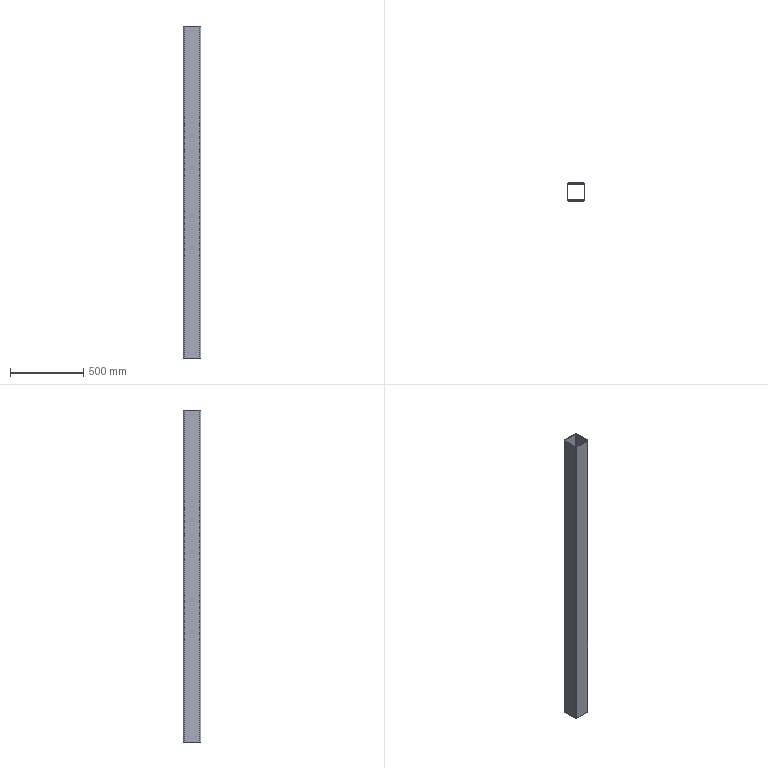Part | SolidWorks | features ICE 1, LibraryFeature 1 | 1 solid | 18 faces | box 120 x 120 x 2260 mm | volume 4101440 mm3 | plane 10 | cylinder 8 | commonest cylinder face diameters 8 x4 16 x4
STEP:
#1=CARTESIAN_POINT('',(52.,60.,-1130.));
#2=VERTEX_POINT('',#1);
#3=CARTESIAN_POINT('',(-52.,60.,-1130.));
#4=VERTEX_POINT('',#3);
#5=CARTESIAN_POINT('',(0.,60.,-1130.));
#6=DIRECTION('',(-1.,0.,0.));
#7=VECTOR('',#6,1000.);
#8=LINE('',#5,#7);
#9=EDGE_CURVE('',#2,#4,#8,.T.);
#10=ORIENTED_EDGE('',*,*,#9,.T.);
#11=CARTESIAN_POINT('',(-52.,60.,1130.));
#12=VERTEX_POINT('',#11);
#13=CARTESIAN_POINT('',(-52.,60.,1130.));
#14=DIRECTION('',(0.,0.,-1.));
#15=VECTOR('',#14,1000.);
#16=LINE('',#13,#15);
#17=EDGE_CURVE('',#12,#4,#16,.T.);
#18=ORIENTED_EDGE('',*,*,#17,.F.);
#19=CARTESIAN_POINT('',(52.,60.,1130.));
#20=VERTEX_POINT('',#19);
#21=CARTESIAN_POINT('',(0.,60.,1130.));
#22=DIRECTION('',(-1.,0.,0.));
#23=VECTOR('',#22,1000.);
#24=LINE('',#21,#23);
#25=EDGE_CURVE('',#20,#12,#24,.T.);
#26=ORIENTED_EDGE('',*,*,#25,.F.);
#27=CARTESIAN_POINT('',(52.,60.,1130.));
#28=DIRECTION('',(0.,0.,-1.));
#29=VECTOR('',#28,1000.);
#30=LINE('',#27,#29);
#31=EDGE_CURVE('',#20,#2,#30,.T.);
#32=ORIENTED_EDGE('',*,*,#31,.T.);
#33=EDGE_LOOP('',(#10,#18,#26,#32));
#34=FACE_OUTER_BOUND('',#33,.T.);
#35=CARTESIAN_POINT('',(0.,60.,1130.));
#36=DIRECTION('',(0.,-1.,0.));
#37=DIRECTION('',(0.,0.,-1.));
#38=AXIS2_PLACEMENT_3D('',#35,#36,#37);
#39=PLANE('',#38);
#40=ADVANCED_FACE('',(#34),#39,.F.);
#41=CARTESIAN_POINT('',(-60.,52.,-1130.));
#42=VERTEX_POINT('',#41);
#43=CARTESIAN_POINT('',(-52.,52.,-1130.));
#44=DIRECTION('',(0.,0.,1.));
#45=DIRECTION('',(1.,0.,0.));
#46=AXIS2_PLACEMENT_3D('',#43,#44,#45);
#47=CIRCLE('',#46,8.);
#48=EDGE_CURVE('',#4,#42,#47,.T.);
#49=ORIENTED_EDGE('',*,*,#48,.T.);
#50=CARTESIAN_POINT('',(-60.,52.,1130.));
#51=VERTEX_POINT('',#50);
#52=CARTESIAN_POINT('',(-60.,52.,1130.));
#53=DIRECTION('',(0.,0.,-1.));
#54=VECTOR('',#53,1000.);
#55=LINE('',#52,#54);
#56=EDGE_CURVE('',#51,#42,#55,.T.);
#57=ORIENTED_EDGE('',*,*,#56,.F.);
#58=CARTESIAN_POINT('',(-52.,52.,1130.));
#59=DIRECTION('',(0.,0.,1.));
#60=DIRECTION('',(1.,0.,0.));
#61=AXIS2_PLACEMENT_3D('',#58,#59,#60);
#62=CIRCLE('',#61,8.);
#63=EDGE_CURVE('',#12,#51,#62,.T.);
#64=ORIENTED_EDGE('',*,*,#63,.F.);
#65=ORIENTED_EDGE('',*,*,#17,.T.);
#66=EDGE_LOOP('',(#49,#57,#64,#65));
#67=FACE_OUTER_BOUND('',#66,.T.);
#68=CARTESIAN_POINT('',(-52.,52.,1130.));
#69=DIRECTION('',(0.,0.,-1.));
#70=DIRECTION('',(-1.,0.,0.));
#71=AXIS2_PLACEMENT_3D('',#68,#69,#70);
#72=CYLINDRICAL_SURFACE('',#71,8.);
#73=ADVANCED_FACE('',(#67),#72,.T.);
#74=CARTESIAN_POINT('',(-60.,-52.,-1130.));
#75=VERTEX_POINT('',#74);
#76=CARTESIAN_POINT('',(-60.,0.,-1130.));
#77=DIRECTION('',(0.,1.,0.));
#78=VECTOR('',#77,1000.);
#79=LINE('',#76,#78);
#80=EDGE_CURVE('',#75,#42,#79,.T.);
#81=ORIENTED_EDGE('',*,*,#80,.F.);
#82=CARTESIAN_POINT('',(-60.,-52.,1130.));
#83=VERTEX_POINT('',#82);
#84=CARTESIAN_POINT('',(-60.,-52.,1130.));
#85=DIRECTION('',(0.,0.,-1.));
#86=VECTOR('',#85,1000.);
#87=LINE('',#84,#86);
#88=EDGE_CURVE('',#83,#75,#87,.T.);
#89=ORIENTED_EDGE('',*,*,#88,.F.);
#90=CARTESIAN_POINT('',(-60.,0.,1130.));
#91=DIRECTION('',(0.,1.,0.));
#92=VECTOR('',#91,1000.);
#93=LINE('',#90,#92);
#94=EDGE_CURVE('',#83,#51,#93,.T.);
#95=ORIENTED_EDGE('',*,*,#94,.T.);
#96=ORIENTED_EDGE('',*,*,#56,.T.);
#97=EDGE_LOOP('',(#81,#89,#95,#96));
#98=FACE_OUTER_BOUND('',#97,.T.);
#99=CARTESIAN_POINT('',(-60.,0.,1130.));
#100=DIRECTION('',(-1.,0.,0.));
#101=DIRECTION('',(0.,0.,1.));
#102=AXIS2_PLACEMENT_3D('',#99,#100,#101);
#103=PLANE('',#102);
#104=ADVANCED_FACE('',(#98),#103,.T.);
#105=CARTESIAN_POINT('',(-52.,-60.,-1130.));
#106=VERTEX_POINT('',#105);
#107=CARTESIAN_POINT('',(-52.,-52.,-1130.));
#108=DIRECTION('',(0.,0.,1.));
#109=DIRECTION('',(1.,0.,0.));
#110=AXIS2_PLACEMENT_3D('',#107,#108,#109);
#111=CIRCLE('',#110,8.);
#112=EDGE_CURVE('',#75,#106,#111,.T.);
#113=ORIENTED_EDGE('',*,*,#112,.T.);
#114=CARTESIAN_POINT('',(-52.,-60.,1130.));
#115=VERTEX_POINT('',#114);
#116=CARTESIAN_POINT('',(-52.,-60.,1130.));
#117=DIRECTION('',(0.,0.,-1.));
#118=VECTOR('',#117,1000.);
#119=LINE('',#116,#118);
#120=EDGE_CURVE('',#115,#106,#119,.T.);
#121=ORIENTED_EDGE('',*,*,#120,.F.);
#122=CARTESIAN_POINT('',(-52.,-52.,1130.));
#123=DIRECTION('',(0.,0.,1.));
#124=DIRECTION('',(1.,0.,0.));
#125=AXIS2_PLACEMENT_3D('',#122,#123,#124);
#126=CIRCLE('',#125,8.);
#127=EDGE_CURVE('',#83,#115,#126,.T.);
#128=ORIENTED_EDGE('',*,*,#127,.F.);
#129=ORIENTED_EDGE('',*,*,#88,.T.);
#130=EDGE_LOOP('',(#113,#121,#128,#129));
#131=FACE_OUTER_BOUND('',#130,.T.);
#132=CARTESIAN_POINT('',(-52.,-52.,1130.));
#133=DIRECTION('',(0.,0.,-1.));
#134=DIRECTION('',(-1.,0.,0.));
#135=AXIS2_PLACEMENT_3D('',#132,#133,#134);
#136=CYLINDRICAL_SURFACE('',#135,8.);
#137=ADVANCED_FACE('',(#131),#136,.T.);
#138=CARTESIAN_POINT('',(52.,-60.,-1130.));
#139=VERTEX_POINT('',#138);
#140=CARTESIAN_POINT('',(0.,-60.,-1130.));
#141=DIRECTION('',(1.,0.,0.));
#142=VECTOR('',#141,1000.);
#143=LINE('',#140,#142);
#144=EDGE_CURVE('',#106,#139,#143,.T.);
#145=ORIENTED_EDGE('',*,*,#144,.T.);
#146=CARTESIAN_POINT('',(52.,-60.,1130.));
#147=VERTEX_POINT('',#146);
#148=CARTESIAN_POINT('',(52.,-60.,1130.));
#149=DIRECTION('',(0.,0.,-1.));
#150=VECTOR('',#149,1000.);
#151=LINE('',#148,#150);
#152=EDGE_CURVE('',#147,#139,#151,.T.);
#153=ORIENTED_EDGE('',*,*,#152,.F.);
#154=CARTESIAN_POINT('',(0.,-60.,1130.));
#155=DIRECTION('',(1.,0.,0.));
#156=VECTOR('',#155,1000.);
#157=LINE('',#154,#156);
#158=EDGE_CURVE('',#115,#147,#157,.T.);
#159=ORIENTED_EDGE('',*,*,#158,.F.);
#160=ORIENTED_EDGE('',*,*,#120,.T.);
#161=EDGE_LOOP('',(#145,#153,#159,#160));
#162=FACE_OUTER_BOUND('',#161,.T.);
#163=CARTESIAN_POINT('',(0.,-60.,1130.));
#164=DIRECTION('',(0.,1.,0.));
#165=DIRECTION('',(0.,0.,1.));
#166=AXIS2_PLACEMENT_3D('',#163,#164,#165);
#167=PLANE('',#166);
#168=ADVANCED_FACE('',(#162),#167,.F.);
#169=CARTESIAN_POINT('',(60.,-52.,-1130.));
#170=VERTEX_POINT('',#169);
#171=CARTESIAN_POINT('',(52.,-52.,-1130.));
#172=DIRECTION('',(0.,0.,1.));
#173=DIRECTION('',(1.,0.,0.));
#174=AXIS2_PLACEMENT_3D('',#171,#172,#173);
#175=CIRCLE('',#174,8.);
#176=EDGE_CURVE('',#139,#170,#175,.T.);
#177=ORIENTED_EDGE('',*,*,#176,.T.);
#178=CARTESIAN_POINT('',(60.,-52.,1130.));
#179=VERTEX_POINT('',#178);
#180=CARTESIAN_POINT('',(60.,-52.,1130.));
#181=DIRECTION('',(0.,0.,-1.));
#182=VECTOR('',#181,1000.);
#183=LINE('',#180,#182);
#184=EDGE_CURVE('',#179,#170,#183,.T.);
#185=ORIENTED_EDGE('',*,*,#184,.F.);
#186=CARTESIAN_POINT('',(52.,-52.,1130.));
#187=DIRECTION('',(0.,0.,1.));
#188=DIRECTION('',(1.,0.,0.));
#189=AXIS2_PLACEMENT_3D('',#186,#187,#188);
#190=CIRCLE('',#189,8.);
#191=EDGE_CURVE('',#147,#179,#190,.T.);
#192=ORIENTED_EDGE('',*,*,#191,.F.);
#193=ORIENTED_EDGE('',*,*,#152,.T.);
#194=EDGE_LOOP('',(#177,#185,#192,#193));
#195=FACE_OUTER_BOUND('',#194,.T.);
#196=CARTESIAN_POINT('',(52.,-52.,1130.));
#197=DIRECTION('',(0.,0.,-1.));
#198=DIRECTION('',(-1.,0.,0.));
#199=AXIS2_PLACEMENT_3D('',#196,#197,#198);
#200=CYLINDRICAL_SURFACE('',#199,8.);
#201=ADVANCED_FACE('',(#195),#200,.T.);
#202=CARTESIAN_POINT('',(60.,52.,-1130.));
#203=VERTEX_POINT('',#202);
#204=CARTESIAN_POINT('',(60.,0.,-1130.));
#205=DIRECTION('',(0.,-1.,0.));
#206=VECTOR('',#205,1000.);
#207=LINE('',#204,#206);
#208=EDGE_CURVE('',#203,#170,#207,.T.);
#209=ORIENTED_EDGE('',*,*,#208,.F.);
#210=CARTESIAN_POINT('',(60.,52.,1130.));
#211=VERTEX_POINT('',#210);
#212=CARTESIAN_POINT('',(60.,52.,1130.));
#213=DIRECTION('',(0.,0.,-1.));
#214=VECTOR('',#213,1000.);
#215=LINE('',#212,#214);
#216=EDGE_CURVE('',#211,#203,#215,.T.);
#217=ORIENTED_EDGE('',*,*,#216,.F.);
#218=CARTESIAN_POINT('',(60.,0.,1130.));
#219=DIRECTION('',(0.,-1.,0.));
#220=VECTOR('',#219,1000.);
#221=LINE('',#218,#220);
#222=EDGE_CURVE('',#211,#179,#221,.T.);
#223=ORIENTED_EDGE('',*,*,#222,.T.);
#224=ORIENTED_EDGE('',*,*,#184,.T.);
#225=EDGE_LOOP('',(#209,#217,#223,#224));
#226=FACE_OUTER_BOUND('',#225,.T.);
#227=CARTESIAN_POINT('',(60.,0.,1130.));
#228=DIRECTION('',(1.,0.,0.));
#229=DIRECTION('',(0.,0.,-1.));
#230=AXIS2_PLACEMENT_3D('',#227,#228,#229);
#231=PLANE('',#230);
#232=ADVANCED_FACE('',(#226),#231,.T.);
#233=CARTESIAN_POINT('',(-56.,-52.,-1130.));
#234=VERTEX_POINT('',#233);
#235=CARTESIAN_POINT('',(-52.,-56.,-1130.));
#236=VERTEX_POINT('',#235);
#237=CARTESIAN_POINT('',(-52.,-52.,-1130.));
#238=DIRECTION('',(0.,0.,1.));
#239=DIRECTION('',(1.,0.,0.));
#240=AXIS2_PLACEMENT_3D('',#237,#238,#239);
#241=CIRCLE('',#240,4.);
#242=EDGE_CURVE('',#234,#236,#241,.T.);
#243=ORIENTED_EDGE('',*,*,#242,.F.);
#244=CARTESIAN_POINT('',(-56.,-52.,1130.));
#245=VERTEX_POINT('',#244);
#246=CARTESIAN_POINT('',(-56.,-52.,1130.));
#247=DIRECTION('',(0.,0.,-1.));
#248=VECTOR('',#247,1000.);
#249=LINE('',#246,#248);
#250=EDGE_CURVE('',#245,#234,#249,.T.);
#251=ORIENTED_EDGE('',*,*,#250,.F.);
#252=CARTESIAN_POINT('',(-52.,-56.,1130.));
#253=VERTEX_POINT('',#252);
#254=CARTESIAN_POINT('',(-52.,-52.,1130.));
#255=DIRECTION('',(0.,0.,1.));
#256=DIRECTION('',(1.,0.,0.));
#257=AXIS2_PLACEMENT_3D('',#254,#255,#256);
#258=CIRCLE('',#257,4.);
#259=EDGE_CURVE('',#245,#253,#258,.T.);
#260=ORIENTED_EDGE('',*,*,#259,.T.);
#261=CARTESIAN_POINT('',(-52.,-56.,1130.));
#262=DIRECTION('',(0.,0.,-1.));
#263=VECTOR('',#262,1000.);
#264=LINE('',#261,#263);
#265=EDGE_CURVE('',#253,#236,#264,.T.);
#266=ORIENTED_EDGE('',*,*,#265,.T.);
#267=EDGE_LOOP('',(#243,#251,#260,#266));
#268=FACE_OUTER_BOUND('',#267,.T.);
#269=CARTESIAN_POINT('',(-52.,-52.,1130.));
#270=DIRECTION('',(0.,0.,-1.));
#271=DIRECTION('',(-1.,0.,0.));
#272=AXIS2_PLACEMENT_3D('',#269,#270,#271);
#273=CYLINDRICAL_SURFACE('',#272,4.);
#274=ADVANCED_FACE('',(#268),#273,.F.);
#275=CARTESIAN_POINT('',(-56.,52.,-1130.));
#276=VERTEX_POINT('',#275);
#277=CARTESIAN_POINT('',(-56.,0.,-1130.));
#278=DIRECTION('',(0.,1.,0.));
#279=VECTOR('',#278,1000.);
#280=LINE('',#277,#279);
#281=EDGE_CURVE('',#234,#276,#280,.T.);
#282=ORIENTED_EDGE('',*,*,#281,.T.);
#283=CARTESIAN_POINT('',(-56.,52.,1130.));
#284=VERTEX_POINT('',#283);
#285=CARTESIAN_POINT('',(-56.,52.,1130.));
#286=DIRECTION('',(0.,0.,-1.));
#287=VECTOR('',#286,1000.);
#288=LINE('',#285,#287);
#289=EDGE_CURVE('',#284,#276,#288,.T.);
#290=ORIENTED_EDGE('',*,*,#289,.F.);
#291=CARTESIAN_POINT('',(-56.,0.,1130.));
#292=DIRECTION('',(0.,1.,0.));
#293=VECTOR('',#292,1000.);
#294=LINE('',#291,#293);
#295=EDGE_CURVE('',#245,#284,#294,.T.);
#296=ORIENTED_EDGE('',*,*,#295,.F.);
#297=ORIENTED_EDGE('',*,*,#250,.T.);
#298=EDGE_LOOP('',(#282,#290,#296,#297));
#299=FACE_OUTER_BOUND('',#298,.T.);
#300=CARTESIAN_POINT('',(-56.,0.,1130.));
#301=DIRECTION('',(-1.,0.,0.));
#302=DIRECTION('',(0.,0.,1.));
#303=AXIS2_PLACEMENT_3D('',#300,#301,#302);
#304=PLANE('',#303);
#305=ADVANCED_FACE('',(#299),#304,.F.);
#306=CARTESIAN_POINT('',(-52.,56.,-1130.));
#307=VERTEX_POINT('',#306);
#308=CARTESIAN_POINT('',(-52.,52.,-1130.));
#309=DIRECTION('',(0.,0.,1.));
#310=DIRECTION('',(1.,0.,0.));
#311=AXIS2_PLACEMENT_3D('',#308,#309,#310);
#312=CIRCLE('',#311,4.);
#313=EDGE_CURVE('',#307,#276,#312,.T.);
#314=ORIENTED_EDGE('',*,*,#313,.F.);
#315=CARTESIAN_POINT('',(-52.,56.,1130.));
#316=VERTEX_POINT('',#315);
#317=CARTESIAN_POINT('',(-52.,56.,1130.));
#318=DIRECTION('',(0.,0.,-1.));
#319=VECTOR('',#318,1000.);
#320=LINE('',#317,#319);
#321=EDGE_CURVE('',#316,#307,#320,.T.);
#322=ORIENTED_EDGE('',*,*,#321,.F.);
#323=CARTESIAN_POINT('',(-52.,52.,1130.));
#324=DIRECTION('',(0.,0.,1.));
#325=DIRECTION('',(1.,0.,0.));
#326=AXIS2_PLACEMENT_3D('',#323,#324,#325);
#327=CIRCLE('',#326,4.);
#328=EDGE_CURVE('',#316,#284,#327,.T.);
#329=ORIENTED_EDGE('',*,*,#328,.T.);
#330=ORIENTED_EDGE('',*,*,#289,.T.);
#331=EDGE_LOOP('',(#314,#322,#329,#330));
#332=FACE_OUTER_BOUND('',#331,.T.);
#333=CARTESIAN_POINT('',(-52.,52.,1130.));
#334=DIRECTION('',(0.,0.,-1.));
#335=DIRECTION('',(-1.,0.,0.));
#336=AXIS2_PLACEMENT_3D('',#333,#334,#335);
#337=CYLINDRICAL_SURFACE('',#336,4.);
#338=ADVANCED_FACE('',(#332),#337,.F.);
#339=CARTESIAN_POINT('',(52.,56.,-1130.));
#340=VERTEX_POINT('',#339);
#341=CARTESIAN_POINT('',(0.,56.,-1130.));
#342=DIRECTION('',(-1.,0.,0.));
#343=VECTOR('',#342,1000.);
#344=LINE('',#341,#343);
#345=EDGE_CURVE('',#340,#307,#344,.T.);
#346=ORIENTED_EDGE('',*,*,#345,.F.);
#347=CARTESIAN_POINT('',(52.,56.,1130.));
#348=VERTEX_POINT('',#347);
#349=CARTESIAN_POINT('',(52.,56.,1130.));
#350=DIRECTION('',(0.,0.,-1.));
#351=VECTOR('',#350,1000.);
#352=LINE('',#349,#351);
#353=EDGE_CURVE('',#348,#340,#352,.T.);
#354=ORIENTED_EDGE('',*,*,#353,.F.);
#355=CARTESIAN_POINT('',(0.,56.,1130.));
#356=DIRECTION('',(-1.,0.,0.));
#357=VECTOR('',#356,1000.);
#358=LINE('',#355,#357);
#359=EDGE_CURVE('',#348,#316,#358,.T.);
#360=ORIENTED_EDGE('',*,*,#359,.T.);
#361=ORIENTED_EDGE('',*,*,#321,.T.);
#362=EDGE_LOOP('',(#346,#354,#360,#361));
#363=FACE_OUTER_BOUND('',#362,.T.);
#364=CARTESIAN_POINT('',(0.,56.,1130.));
#365=DIRECTION('',(0.,-1.,0.));
#366=DIRECTION('',(0.,0.,-1.));
#367=AXIS2_PLACEMENT_3D('',#364,#365,#366);
#368=PLANE('',#367);
#369=ADVANCED_FACE('',(#363),#368,.T.);
#370=CARTESIAN_POINT('',(56.,52.,-1130.));
#371=VERTEX_POINT('',#370);
#372=CARTESIAN_POINT('',(52.,52.,-1130.));
#373=DIRECTION('',(0.,0.,1.));
#374=DIRECTION('',(1.,0.,0.));
#375=AXIS2_PLACEMENT_3D('',#372,#373,#374);
#376=CIRCLE('',#375,4.);
#377=EDGE_CURVE('',#371,#340,#376,.T.);
#378=ORIENTED_EDGE('',*,*,#377,.F.);
#379=CARTESIAN_POINT('',(56.,52.,1130.));
#380=VERTEX_POINT('',#379);
#381=CARTESIAN_POINT('',(56.,52.,1130.));
#382=DIRECTION('',(0.,0.,-1.));
#383=VECTOR('',#382,1000.);
#384=LINE('',#381,#383);
#385=EDGE_CURVE('',#380,#371,#384,.T.);
#386=ORIENTED_EDGE('',*,*,#385,.F.);
#387=CARTESIAN_POINT('',(52.,52.,1130.));
#388=DIRECTION('',(0.,0.,1.));
#389=DIRECTION('',(1.,0.,0.));
#390=AXIS2_PLACEMENT_3D('',#387,#388,#389);
#391=CIRCLE('',#390,4.);
#392=EDGE_CURVE('',#380,#348,#391,.T.);
#393=ORIENTED_EDGE('',*,*,#392,.T.);
#394=ORIENTED_EDGE('',*,*,#353,.T.);
#395=EDGE_LOOP('',(#378,#386,#393,#394));
#396=FACE_OUTER_BOUND('',#395,.T.);
#397=CARTESIAN_POINT('',(52.,52.,1130.));
#398=DIRECTION('',(0.,0.,-1.));
#399=DIRECTION('',(-1.,0.,0.));
#400=AXIS2_PLACEMENT_3D('',#397,#398,#399);
#401=CYLINDRICAL_SURFACE('',#400,4.);
#402=ADVANCED_FACE('',(#396),#401,.F.);
#403=CARTESIAN_POINT('',(56.,-52.,-1130.));
#404=VERTEX_POINT('',#403);
#405=CARTESIAN_POINT('',(56.,0.,-1130.));
#406=DIRECTION('',(0.,-1.,0.));
#407=VECTOR('',#406,1000.);
#408=LINE('',#405,#407);
#409=EDGE_CURVE('',#371,#404,#408,.T.);
#410=ORIENTED_EDGE('',*,*,#409,.T.);
#411=CARTESIAN_POINT('',(56.,-52.,1130.));
#412=VERTEX_POINT('',#411);
#413=CARTESIAN_POINT('',(56.,-52.,1130.));
#414=DIRECTION('',(0.,0.,-1.));
#415=VECTOR('',#414,1000.);
#416=LINE('',#413,#415);
#417=EDGE_CURVE('',#412,#404,#416,.T.);
#418=ORIENTED_EDGE('',*,*,#417,.F.);
#419=CARTESIAN_POINT('',(56.,0.,1130.));
#420=DIRECTION('',(0.,-1.,0.));
#421=VECTOR('',#420,1000.);
#422=LINE('',#419,#421);
#423=EDGE_CURVE('',#380,#412,#422,.T.);
#424=ORIENTED_EDGE('',*,*,#423,.F.);
#425=ORIENTED_EDGE('',*,*,#385,.T.);
#426=EDGE_LOOP('',(#410,#418,#424,#425));
#427=FACE_OUTER_BOUND('',#426,.T.);
#428=CARTESIAN_POINT('',(56.,0.,1130.));
#429=DIRECTION('',(1.,0.,0.));
#430=DIRECTION('',(0.,0.,-1.));
#431=AXIS2_PLACEMENT_3D('',#428,#429,#430);
#432=PLANE('',#431);
#433=ADVANCED_FACE('',(#427),#432,.F.);
#434=CARTESIAN_POINT('',(52.,-56.,-1130.));
#435=VERTEX_POINT('',#434);
#436=CARTESIAN_POINT('',(52.,-52.,-1130.));
#437=DIRECTION('',(0.,0.,1.));
#438=DIRECTION('',(1.,0.,0.));
#439=AXIS2_PLACEMENT_3D('',#436,#437,#438);
#440=CIRCLE('',#439,4.);
#441=EDGE_CURVE('',#435,#404,#440,.T.);
#442=ORIENTED_EDGE('',*,*,#441,.F.);
#443=CARTESIAN_POINT('',(52.,-56.,1130.));
#444=VERTEX_POINT('',#443);
#445=CARTESIAN_POINT('',(52.,-56.,1130.));
#446=DIRECTION('',(0.,0.,-1.));
#447=VECTOR('',#446,1000.);
#448=LINE('',#445,#447);
#449=EDGE_CURVE('',#444,#435,#448,.T.);
#450=ORIENTED_EDGE('',*,*,#449,.F.);
#451=CARTESIAN_POINT('',(52.,-52.,1130.));
#452=DIRECTION('',(0.,0.,1.));
#453=DIRECTION('',(1.,0.,0.));
#454=AXIS2_PLACEMENT_3D('',#451,#452,#453);
#455=CIRCLE('',#454,4.);
#456=EDGE_CURVE('',#444,#412,#455,.T.);
#457=ORIENTED_EDGE('',*,*,#456,.T.);
#458=ORIENTED_EDGE('',*,*,#417,.T.);
#459=EDGE_LOOP('',(#442,#450,#457,#458));
#460=FACE_OUTER_BOUND('',#459,.T.);
#461=CARTESIAN_POINT('',(52.,-52.,1130.));
#462=DIRECTION('',(0.,0.,-1.));
#463=DIRECTION('',(-1.,0.,0.));
#464=AXIS2_PLACEMENT_3D('',#461,#462,#463);
#465=CYLINDRICAL_SURFACE('',#464,4.);
#466=ADVANCED_FACE('',(#460),#465,.F.);
#467=CARTESIAN_POINT('',(0.,-56.,-1130.));
#468=DIRECTION('',(1.,0.,0.));
#469=VECTOR('',#468,1000.);
#470=LINE('',#467,#469);
#471=EDGE_CURVE('',#236,#435,#470,.T.);
#472=ORIENTED_EDGE('',*,*,#471,.F.);
#473=ORIENTED_EDGE('',*,*,#265,.F.);
#474=CARTESIAN_POINT('',(0.,-56.,1130.));
#475=DIRECTION('',(1.,0.,0.));
#476=VECTOR('',#475,1000.);
#477=LINE('',#474,#476);
#478=EDGE_CURVE('',#253,#444,#477,.T.);
#479=ORIENTED_EDGE('',*,*,#478,.T.);
#480=ORIENTED_EDGE('',*,*,#449,.T.);
#481=EDGE_LOOP('',(#472,#473,#479,#480));
#482=FACE_OUTER_BOUND('',#481,.T.);
#483=CARTESIAN_POINT('',(0.,-56.,1130.));
#484=DIRECTION('',(0.,1.,0.));
#485=DIRECTION('',(0.,0.,1.));
#486=AXIS2_PLACEMENT_3D('',#483,#484,#485);
#487=PLANE('',#486);
#488=ADVANCED_FACE('',(#482),#487,.T.);
#489=CARTESIAN_POINT('',(52.,52.,-1130.));
#490=DIRECTION('',(0.,0.,1.));
#491=DIRECTION('',(1.,0.,0.));
#492=AXIS2_PLACEMENT_3D('',#489,#490,#491);
#493=CIRCLE('',#492,8.);
#494=EDGE_CURVE('',#203,#2,#493,.T.);
#495=ORIENTED_EDGE('',*,*,#494,.T.);
#496=ORIENTED_EDGE('',*,*,#31,.F.);
#497=CARTESIAN_POINT('',(52.,52.,1130.));
#498=DIRECTION('',(0.,0.,1.));
#499=DIRECTION('',(1.,0.,0.));
#500=AXIS2_PLACEMENT_3D('',#497,#498,#499);
#501=CIRCLE('',#500,8.);
#502=EDGE_CURVE('',#211,#20,#501,.T.);
#503=ORIENTED_EDGE('',*,*,#502,.F.);
#504=ORIENTED_EDGE('',*,*,#216,.T.);
#505=EDGE_LOOP('',(#495,#496,#503,#504));
#506=FACE_OUTER_BOUND('',#505,.T.);
#507=CARTESIAN_POINT('',(52.,52.,1130.));
#508=DIRECTION('',(0.,0.,-1.));
#509=DIRECTION('',(-1.,0.,0.));
#510=AXIS2_PLACEMENT_3D('',#507,#508,#509);
#511=CYLINDRICAL_SURFACE('',#510,8.);
#512=ADVANCED_FACE('',(#506),#511,.T.);
#513=ORIENTED_EDGE('',*,*,#259,.F.);
#514=ORIENTED_EDGE('',*,*,#295,.T.);
#515=ORIENTED_EDGE('',*,*,#328,.F.);
#516=ORIENTED_EDGE('',*,*,#359,.F.);
#517=ORIENTED_EDGE('',*,*,#392,.F.);
#518=ORIENTED_EDGE('',*,*,#423,.T.);
#519=ORIENTED_EDGE('',*,*,#456,.F.);
#520=ORIENTED_EDGE('',*,*,#478,.F.);
#521=EDGE_LOOP('',(#513,#514,#515,#516,#517,#518,#519,#520));
#522=FACE_BOUND('',#521,.T.);
#523=ORIENTED_EDGE('',*,*,#25,.T.);
#524=ORIENTED_EDGE('',*,*,#63,.T.);
#525=ORIENTED_EDGE('',*,*,#94,.F.);
#526=ORIENTED_EDGE('',*,*,#127,.T.);
#527=ORIENTED_EDGE('',*,*,#158,.T.);
#528=ORIENTED_EDGE('',*,*,#191,.T.);
#529=ORIENTED_EDGE('',*,*,#222,.F.);
#530=ORIENTED_EDGE('',*,*,#502,.T.);
#531=EDGE_LOOP('',(#523,#524,#525,#526,#527,#528,#529,#530));
#532=FACE_OUTER_BOUND('',#531,.T.);
#533=CARTESIAN_POINT('',(0.,0.,1130.));
#534=DIRECTION('',(0.,0.,1.));
#535=DIRECTION('',(1.,0.,0.));
#536=AXIS2_PLACEMENT_3D('',#533,#534,#535);
#537=PLANE('',#536);
#538=ADVANCED_FACE('',(#522,#532),#537,.T.);
#539=ORIENTED_EDGE('',*,*,#242,.T.);
#540=ORIENTED_EDGE('',*,*,#471,.T.);
#541=ORIENTED_EDGE('',*,*,#441,.T.);
#542=ORIENTED_EDGE('',*,*,#409,.F.);
#543=ORIENTED_EDGE('',*,*,#377,.T.);
#544=ORIENTED_EDGE('',*,*,#345,.T.);
#545=ORIENTED_EDGE('',*,*,#313,.T.);
#546=ORIENTED_EDGE('',*,*,#281,.F.);
#547=EDGE_LOOP('',(#539,#540,#541,#542,#543,#544,#545,#546));
#548=FACE_BOUND('',#547,.T.);
#549=ORIENTED_EDGE('',*,*,#9,.F.);
#550=ORIENTED_EDGE('',*,*,#494,.F.);
#551=ORIENTED_EDGE('',*,*,#208,.T.);
#552=ORIENTED_EDGE('',*,*,#176,.F.);
#553=ORIENTED_EDGE('',*,*,#144,.F.);
#554=ORIENTED_EDGE('',*,*,#112,.F.);
#555=ORIENTED_EDGE('',*,*,#80,.T.);
#556=ORIENTED_EDGE('',*,*,#48,.F.);
#557=EDGE_LOOP('',(#549,#550,#551,#552,#553,#554,#555,#556));
#558=FACE_OUTER_BOUND('',#557,.T.);
#559=CARTESIAN_POINT('',(0.,0.,-1130.));
#560=DIRECTION('',(0.,0.,1.));
#561=DIRECTION('',(1.,0.,0.));
#562=AXIS2_PLACEMENT_3D('',#559,#560,#561);
#563=PLANE('',#562);
#564=ADVANCED_FACE('',(#548,#558),#563,.F.);
#565=CLOSED_SHELL('',(#40,#73,#104,#137,#168,#201,#232,#274,#305,#338,#369,#402,#433,#466,#488,#512,#538,#564));
#566=MANIFOLD_SOLID_BREP('',#565);
#567=CARTESIAN_POINT('',(0.,0.,0.));
#568=DIRECTION('',(0.,0.,1.));
#569=DIRECTION('',(1.,0.,0.));
#570=AXIS2_PLACEMENT_3D('',#567,#568,#569);
#571=(LENGTH_UNIT()NAMED_UNIT(*)SI_UNIT(.MILLI.,.METRE.));
#572=UNCERTAINTY_MEASURE_WITH_UNIT(LENGTH_MEASURE(0.00001),#571,'','');
#573=(NAMED_UNIT(*)PLANE_ANGLE_UNIT()SI_UNIT($,.RADIAN.));
#574=(NAMED_UNIT(*)SI_UNIT($,.STERADIAN.)SOLID_ANGLE_UNIT());
#575=(GEOMETRIC_REPRESENTATION_CONTEXT(3)GLOBAL_UNCERTAINTY_ASSIGNED_CONTEXT((#572))GLOBAL_UNIT_ASSIGNED_CONTEXT((#571,#573,#574))REPRESENTATION_CONTEXT('',''));
#576=ADVANCED_BREP_SHAPE_REPRESENTATION('',(#566,#570),#575);